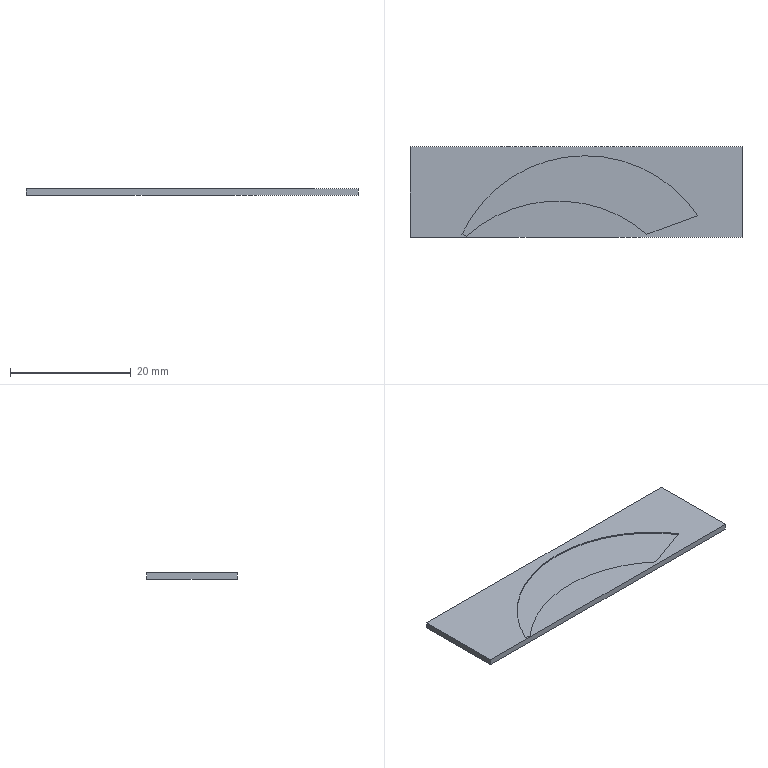Part | STEP file | HXGR200008-06-02-08 | 1 solid | 11 faces | box 55 x 15 x 1 mm | volume 774.16 mm3 | plane 9 | cylinder 2 | commonest cylinder face diameters 45 x2
STEP:
#1=CARTESIAN_POINT('',(27.5,-7.5,0.));
#2=VERTEX_POINT('',#1);
#3=CARTESIAN_POINT('',(27.5,7.5,0.));
#4=VERTEX_POINT('',#3);
#5=CARTESIAN_POINT('',(27.5,7.5,0.));
#6=DIRECTION('',(0.,1.,0.));
#7=VECTOR('',#6,1000.);
#8=LINE('',#5,#7);
#9=EDGE_CURVE('',#2,#4,#8,.T.);
#10=ORIENTED_EDGE('',*,*,#9,.F.);
#11=CARTESIAN_POINT('',(27.5,-7.5,-1.));
#12=VERTEX_POINT('',#11);
#13=CARTESIAN_POINT('',(27.5,-7.5,-1.));
#14=DIRECTION('',(0.,0.,1.));
#15=VECTOR('',#14,1000.);
#16=LINE('',#13,#15);
#17=EDGE_CURVE('',#12,#2,#16,.T.);
#18=ORIENTED_EDGE('',*,*,#17,.F.);
#19=CARTESIAN_POINT('',(27.5,7.5,-1.));
#20=VERTEX_POINT('',#19);
#21=CARTESIAN_POINT('',(27.5,7.5,-1.));
#22=DIRECTION('',(0.,1.,0.));
#23=VECTOR('',#22,1000.);
#24=LINE('',#21,#23);
#25=EDGE_CURVE('',#12,#20,#24,.T.);
#26=ORIENTED_EDGE('',*,*,#25,.T.);
#27=CARTESIAN_POINT('',(27.5,7.5,-1.));
#28=DIRECTION('',(0.,0.,1.));
#29=VECTOR('',#28,1000.);
#30=LINE('',#27,#29);
#31=EDGE_CURVE('',#20,#4,#30,.T.);
#32=ORIENTED_EDGE('',*,*,#31,.T.);
#33=EDGE_LOOP('',(#10,#18,#26,#32));
#34=FACE_OUTER_BOUND('',#33,.T.);
#35=CARTESIAN_POINT('',(27.5,7.5,-1.));
#36=DIRECTION('',(1.,0.,0.));
#37=DIRECTION('',(0.,1.,0.));
#38=AXIS2_PLACEMENT_3D('',#35,#36,#37);
#39=PLANE('',#38);
#40=ADVANCED_FACE('',(#34),#39,.T.);
#41=CARTESIAN_POINT('',(-27.5,-7.5,0.));
#42=VERTEX_POINT('',#41);
#43=CARTESIAN_POINT('',(-27.5,-7.5,0.));
#44=DIRECTION('',(1.,0.,0.));
#45=VECTOR('',#44,1000.);
#46=LINE('',#43,#45);
#47=EDGE_CURVE('',#42,#2,#46,.T.);
#48=ORIENTED_EDGE('',*,*,#47,.F.);
#49=CARTESIAN_POINT('',(-27.5,-7.5,-1.));
#50=VERTEX_POINT('',#49);
#51=CARTESIAN_POINT('',(-27.5,-7.5,-1.));
#52=DIRECTION('',(0.,0.,1.));
#53=VECTOR('',#52,1000.);
#54=LINE('',#51,#53);
#55=EDGE_CURVE('',#50,#42,#54,.T.);
#56=ORIENTED_EDGE('',*,*,#55,.F.);
#57=CARTESIAN_POINT('',(-27.5,-7.5,-1.));
#58=DIRECTION('',(1.,0.,0.));
#59=VECTOR('',#58,1000.);
#60=LINE('',#57,#59);
#61=EDGE_CURVE('',#50,#12,#60,.T.);
#62=ORIENTED_EDGE('',*,*,#61,.T.);
#63=ORIENTED_EDGE('',*,*,#17,.T.);
#64=EDGE_LOOP('',(#48,#56,#62,#63));
#65=FACE_OUTER_BOUND('',#64,.T.);
#66=CARTESIAN_POINT('',(-27.5,-7.5,-1.));
#67=DIRECTION('',(0.,-1.,0.));
#68=DIRECTION('',(0.,0.,-1.));
#69=AXIS2_PLACEMENT_3D('',#66,#67,#68);
#70=PLANE('',#69);
#71=ADVANCED_FACE('',(#65),#70,.T.);
#72=CARTESIAN_POINT('',(-27.5,7.5,0.));
#73=VERTEX_POINT('',#72);
#74=CARTESIAN_POINT('',(-27.5,7.5,0.));
#75=DIRECTION('',(0.,-1.,0.));
#76=VECTOR('',#75,1000.);
#77=LINE('',#74,#76);
#78=EDGE_CURVE('',#73,#42,#77,.T.);
#79=ORIENTED_EDGE('',*,*,#78,.F.);
#80=CARTESIAN_POINT('',(-27.5,7.5,-1.));
#81=VERTEX_POINT('',#80);
#82=CARTESIAN_POINT('',(-27.5,7.5,-1.));
#83=DIRECTION('',(0.,0.,1.));
#84=VECTOR('',#83,1000.);
#85=LINE('',#82,#84);
#86=EDGE_CURVE('',#81,#73,#85,.T.);
#87=ORIENTED_EDGE('',*,*,#86,.F.);
#88=CARTESIAN_POINT('',(-27.5,7.5,-1.));
#89=DIRECTION('',(0.,-1.,0.));
#90=VECTOR('',#89,1000.);
#91=LINE('',#88,#90);
#92=EDGE_CURVE('',#81,#50,#91,.T.);
#93=ORIENTED_EDGE('',*,*,#92,.T.);
#94=ORIENTED_EDGE('',*,*,#55,.T.);
#95=EDGE_LOOP('',(#79,#87,#93,#94));
#96=FACE_OUTER_BOUND('',#95,.T.);
#97=CARTESIAN_POINT('',(-27.5,7.5,-1.));
#98=DIRECTION('',(-1.,0.,0.));
#99=DIRECTION('',(0.,-1.,0.));
#100=AXIS2_PLACEMENT_3D('',#97,#98,#99);
#101=PLANE('',#100);
#102=ADVANCED_FACE('',(#96),#101,.T.);
#103=CARTESIAN_POINT('',(-27.5,7.5,0.));
#104=DIRECTION('',(-1.,0.,0.));
#105=VECTOR('',#104,1000.);
#106=LINE('',#103,#105);
#107=EDGE_CURVE('',#4,#73,#106,.T.);
#108=ORIENTED_EDGE('',*,*,#107,.F.);
#109=ORIENTED_EDGE('',*,*,#31,.F.);
#110=CARTESIAN_POINT('',(-27.5,7.5,-1.));
#111=DIRECTION('',(-1.,0.,0.));
#112=VECTOR('',#111,1000.);
#113=LINE('',#110,#112);
#114=EDGE_CURVE('',#20,#81,#113,.T.);
#115=ORIENTED_EDGE('',*,*,#114,.T.);
#116=ORIENTED_EDGE('',*,*,#86,.T.);
#117=EDGE_LOOP('',(#108,#109,#115,#116));
#118=FACE_OUTER_BOUND('',#117,.T.);
#119=CARTESIAN_POINT('',(-27.5,7.5,-1.));
#120=DIRECTION('',(0.,1.,0.));
#121=DIRECTION('',(0.,0.,1.));
#122=AXIS2_PLACEMENT_3D('',#119,#120,#121);
#123=PLANE('',#122);
#124=ADVANCED_FACE('',(#118),#123,.T.);
#125=ORIENTED_EDGE('',*,*,#25,.F.);
#126=ORIENTED_EDGE('',*,*,#61,.F.);
#127=ORIENTED_EDGE('',*,*,#92,.F.);
#128=ORIENTED_EDGE('',*,*,#114,.F.);
#129=EDGE_LOOP('',(#125,#126,#127,#128));
#130=FACE_OUTER_BOUND('',#129,.T.);
#131=CARTESIAN_POINT('',(0.,0.,-1.));
#132=DIRECTION('',(0.,0.,1.));
#133=DIRECTION('',(1.,0.,0.));
#134=AXIS2_PLACEMENT_3D('',#131,#132,#133);
#135=PLANE('',#134);
#136=ADVANCED_FACE('',(#130),#135,.F.);
#137=CARTESIAN_POINT('',(-18.13,-7.346,0.));
#138=VERTEX_POINT('',#137);
#139=CARTESIAN_POINT('',(11.739,-7.,0.));
#140=VERTEX_POINT('',#139);
#141=CARTESIAN_POINT('',(-3.,-24.,0.));
#142=DIRECTION('',(0.,0.,-1.));
#143=DIRECTION('',(1.,0.,0.));
#144=AXIS2_PLACEMENT_3D('',#141,#142,#143);
#145=CIRCLE('',#144,22.5);
#146=EDGE_CURVE('',#138,#140,#145,.T.);
#147=ORIENTED_EDGE('',*,*,#146,.F.);
#148=CARTESIAN_POINT('',(-18.892,-6.991,0.));
#149=VERTEX_POINT('',#148);
#150=CARTESIAN_POINT('',(-18.13,-7.346,0.));
#151=DIRECTION('',(0.9063,-0.4226,0.));
#152=VECTOR('',#151,1000.);
#153=LINE('',#150,#152);
#154=EDGE_CURVE('',#149,#138,#153,.T.);
#155=ORIENTED_EDGE('',*,*,#154,.F.);
#156=CARTESIAN_POINT('',(20.164,-3.934,0.));
#157=VERTEX_POINT('',#156);
#158=CARTESIAN_POINT('',(1.5,-16.5,0.));
#159=DIRECTION('',(0.,0.,1.));
#160=DIRECTION('',(1.,0.,0.));
#161=AXIS2_PLACEMENT_3D('',#158,#159,#160);
#162=CIRCLE('',#161,22.5);
#163=EDGE_CURVE('',#157,#149,#162,.T.);
#164=ORIENTED_EDGE('',*,*,#163,.F.);
#165=CARTESIAN_POINT('',(11.739,-7.,0.));
#166=DIRECTION('',(0.9397,0.342,0.));
#167=VECTOR('',#166,1000.);
#168=LINE('',#165,#167);
#169=EDGE_CURVE('',#140,#157,#168,.T.);
#170=ORIENTED_EDGE('',*,*,#169,.F.);
#171=EDGE_LOOP('',(#147,#155,#164,#170));
#172=FACE_BOUND('',#171,.T.);
#173=ORIENTED_EDGE('',*,*,#9,.T.);
#174=ORIENTED_EDGE('',*,*,#107,.T.);
#175=ORIENTED_EDGE('',*,*,#78,.T.);
#176=ORIENTED_EDGE('',*,*,#47,.T.);
#177=EDGE_LOOP('',(#173,#174,#175,#176));
#178=FACE_OUTER_BOUND('',#177,.T.);
#179=CARTESIAN_POINT('',(0.,0.,0.));
#180=DIRECTION('',(0.,0.,1.));
#181=DIRECTION('',(1.,0.,0.));
#182=AXIS2_PLACEMENT_3D('',#179,#180,#181);
#183=PLANE('',#182);
#184=ADVANCED_FACE('',(#172,#178),#183,.T.);
#185=ORIENTED_EDGE('',*,*,#146,.T.);
#186=CARTESIAN_POINT('',(11.739,-7.,-0.2));
#187=VERTEX_POINT('',#186);
#188=CARTESIAN_POINT('',(11.739,-7.,-0.2));
#189=DIRECTION('',(0.,0.,1.));
#190=VECTOR('',#189,1000.);
#191=LINE('',#188,#190);
#192=EDGE_CURVE('',#187,#140,#191,.T.);
#193=ORIENTED_EDGE('',*,*,#192,.F.);
#194=CARTESIAN_POINT('',(-18.13,-7.346,-0.2));
#195=VERTEX_POINT('',#194);
#196=CARTESIAN_POINT('',(-3.,-24.,-0.2));
#197=DIRECTION('',(0.,0.,-1.));
#198=DIRECTION('',(1.,0.,0.));
#199=AXIS2_PLACEMENT_3D('',#196,#197,#198);
#200=CIRCLE('',#199,22.5);
#201=EDGE_CURVE('',#195,#187,#200,.T.);
#202=ORIENTED_EDGE('',*,*,#201,.F.);
#203=CARTESIAN_POINT('',(-18.13,-7.346,-0.2));
#204=DIRECTION('',(0.,0.,1.));
#205=VECTOR('',#204,1000.);
#206=LINE('',#203,#205);
#207=EDGE_CURVE('',#195,#138,#206,.T.);
#208=ORIENTED_EDGE('',*,*,#207,.T.);
#209=EDGE_LOOP('',(#185,#193,#202,#208));
#210=FACE_OUTER_BOUND('',#209,.T.);
#211=CARTESIAN_POINT('',(-3.,-24.,-0.2));
#212=DIRECTION('',(0.,0.,1.));
#213=DIRECTION('',(1.,0.,0.));
#214=AXIS2_PLACEMENT_3D('',#211,#212,#213);
#215=CYLINDRICAL_SURFACE('',#214,22.5);
#216=ADVANCED_FACE('',(#210),#215,.T.);
#217=ORIENTED_EDGE('',*,*,#154,.T.);
#218=ORIENTED_EDGE('',*,*,#207,.F.);
#219=CARTESIAN_POINT('',(-18.892,-6.991,-0.2));
#220=VERTEX_POINT('',#219);
#221=CARTESIAN_POINT('',(-18.13,-7.346,-0.2));
#222=DIRECTION('',(0.9063,-0.4226,0.));
#223=VECTOR('',#222,1000.);
#224=LINE('',#221,#223);
#225=EDGE_CURVE('',#220,#195,#224,.T.);
#226=ORIENTED_EDGE('',*,*,#225,.F.);
#227=CARTESIAN_POINT('',(-18.892,-6.991,-0.2));
#228=DIRECTION('',(0.,0.,1.));
#229=VECTOR('',#228,1000.);
#230=LINE('',#227,#229);
#231=EDGE_CURVE('',#220,#149,#230,.T.);
#232=ORIENTED_EDGE('',*,*,#231,.T.);
#233=EDGE_LOOP('',(#217,#218,#226,#232));
#234=FACE_OUTER_BOUND('',#233,.T.);
#235=CARTESIAN_POINT('',(-18.13,-7.346,-0.2));
#236=DIRECTION('',(-0.4226,-0.9063,0.));
#237=DIRECTION('',(0.9063,-0.4226,0.));
#238=AXIS2_PLACEMENT_3D('',#235,#236,#237);
#239=PLANE('',#238);
#240=ADVANCED_FACE('',(#234),#239,.F.);
#241=ORIENTED_EDGE('',*,*,#163,.T.);
#242=ORIENTED_EDGE('',*,*,#231,.F.);
#243=CARTESIAN_POINT('',(20.164,-3.934,-0.2));
#244=VERTEX_POINT('',#243);
#245=CARTESIAN_POINT('',(1.5,-16.5,-0.2));
#246=DIRECTION('',(0.,0.,1.));
#247=DIRECTION('',(1.,0.,0.));
#248=AXIS2_PLACEMENT_3D('',#245,#246,#247);
#249=CIRCLE('',#248,22.5);
#250=EDGE_CURVE('',#244,#220,#249,.T.);
#251=ORIENTED_EDGE('',*,*,#250,.F.);
#252=CARTESIAN_POINT('',(20.164,-3.934,-0.2));
#253=DIRECTION('',(0.,0.,1.));
#254=VECTOR('',#253,1000.);
#255=LINE('',#252,#254);
#256=EDGE_CURVE('',#244,#157,#255,.T.);
#257=ORIENTED_EDGE('',*,*,#256,.T.);
#258=EDGE_LOOP('',(#241,#242,#251,#257));
#259=FACE_OUTER_BOUND('',#258,.T.);
#260=CARTESIAN_POINT('',(1.5,-16.5,-0.2));
#261=DIRECTION('',(0.,0.,1.));
#262=DIRECTION('',(1.,0.,0.));
#263=AXIS2_PLACEMENT_3D('',#260,#261,#262);
#264=CYLINDRICAL_SURFACE('',#263,22.5);
#265=ADVANCED_FACE('',(#259),#264,.F.);
#266=ORIENTED_EDGE('',*,*,#169,.T.);
#267=ORIENTED_EDGE('',*,*,#256,.F.);
#268=CARTESIAN_POINT('',(11.739,-7.,-0.2));
#269=DIRECTION('',(0.9397,0.342,0.));
#270=VECTOR('',#269,1000.);
#271=LINE('',#268,#270);
#272=EDGE_CURVE('',#187,#244,#271,.T.);
#273=ORIENTED_EDGE('',*,*,#272,.F.);
#274=ORIENTED_EDGE('',*,*,#192,.T.);
#275=EDGE_LOOP('',(#266,#267,#273,#274));
#276=FACE_OUTER_BOUND('',#275,.T.);
#277=CARTESIAN_POINT('',(11.739,-7.,-0.2));
#278=DIRECTION('',(0.342,-0.9397,0.));
#279=DIRECTION('',(0.9397,0.342,0.));
#280=AXIS2_PLACEMENT_3D('',#277,#278,#279);
#281=PLANE('',#280);
#282=ADVANCED_FACE('',(#276),#281,.F.);
#283=ORIENTED_EDGE('',*,*,#201,.T.);
#284=ORIENTED_EDGE('',*,*,#272,.T.);
#285=ORIENTED_EDGE('',*,*,#250,.T.);
#286=ORIENTED_EDGE('',*,*,#225,.T.);
#287=EDGE_LOOP('',(#283,#284,#285,#286));
#288=FACE_OUTER_BOUND('',#287,.T.);
#289=CARTESIAN_POINT('',(-3.,-24.,-0.2));
#290=DIRECTION('',(0.,0.,1.));
#291=DIRECTION('',(1.,0.,0.));
#292=AXIS2_PLACEMENT_3D('',#289,#290,#291);
#293=PLANE('',#292);
#294=ADVANCED_FACE('',(#288),#293,.T.);
#295=CLOSED_SHELL('',(#40,#71,#102,#124,#136,#184,#216,#240,#265,#282,#294));
#296=MANIFOLD_SOLID_BREP('',#295);
#297=CARTESIAN_POINT('',(0.,0.,0.));
#298=DIRECTION('',(0.,0.,1.));
#299=DIRECTION('',(1.,0.,0.));
#300=AXIS2_PLACEMENT_3D('',#297,#298,#299);
#301=(LENGTH_UNIT()NAMED_UNIT(*)SI_UNIT(.MILLI.,.METRE.));
#302=UNCERTAINTY_MEASURE_WITH_UNIT(LENGTH_MEASURE(0.00001),#301,'','');
#303=(NAMED_UNIT(*)PLANE_ANGLE_UNIT()SI_UNIT($,.RADIAN.));
#304=(NAMED_UNIT(*)SI_UNIT($,.STERADIAN.)SOLID_ANGLE_UNIT());
#305=(GEOMETRIC_REPRESENTATION_CONTEXT(3)GLOBAL_UNCERTAINTY_ASSIGNED_CONTEXT((#302))GLOBAL_UNIT_ASSIGNED_CONTEXT((#301,#303,#304))REPRESENTATION_CONTEXT('',''));
#306=ADVANCED_BREP_SHAPE_REPRESENTATION('',(#296,#300),#305);